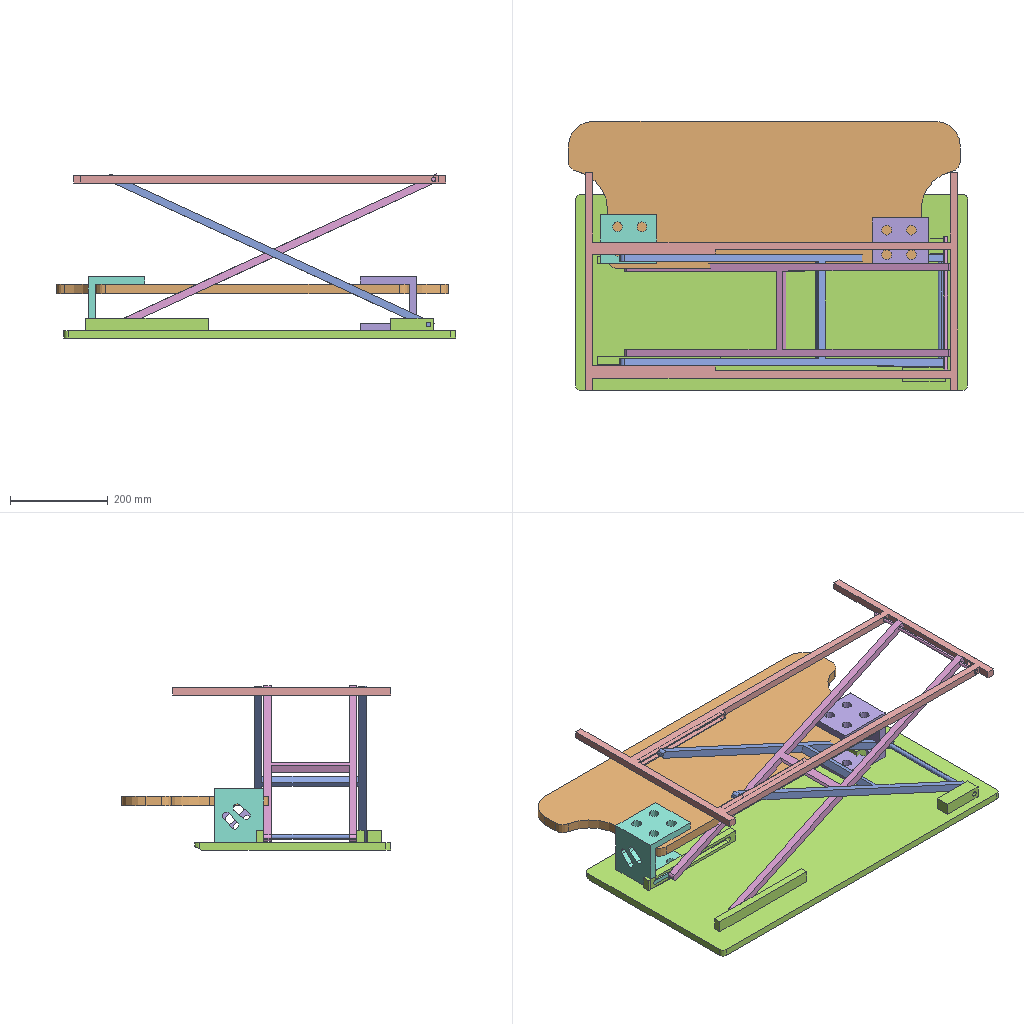Assembly | SolidWorks | 8 different items | 8 placed | box 815 x 549 x 335 mm
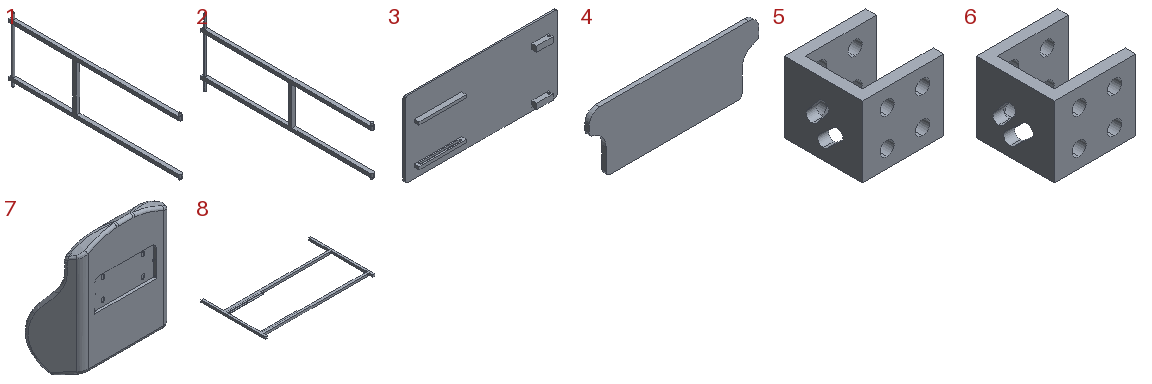Parts list (item | quantity | size | volume | features):
1 | x1 | 15 x 730 x 270 mm | 392693 mm3 | features ICE 5, Extrusion 1, Fillet 1
2 | x1 | 15 x 730 x 285 mm | 378111 mm3 | features ICE 5, Extrusion 1, Fillet 1
3 | x1 | 800 x 40 x 400.131 mm | 4882709 mm3 | features ICE 4, Cut 2, Fillet 2, MirrorPattern 2, Draft 1, Extrusion 1
4 | x1 | 800 x 20 x 300 mm | 4187582 mm3 | features Fillet 2, Extrusion 1
5 | x1 | 115 x 110 x 100 mm | 409059 mm3 | features ICE 2, Extrusion 1
6 | x1 | 115 x 110 x 100 mm | 406186 mm3 | features ICE 2, Extrusion 1
7 | x1 | 1267 x 391.764 x 1203 mm | 196548846 mm3 | features ICE 13, MirrorPattern 6, Fillet 5, Extrusion 1, RefAxis 1, Scale 1
8 | x1 | 760 x 445 x 15 mm | 540712 mm3 | features ICE 4, Cut 1, Extrusion 1
Mates (type | each side: item.copy, entity, surface, feature):
Parallel | 8.1 face plane Boss-Extrude1 | 3.1 face plane Boss-Extrude1
Width | 3.1 face plane Boss-Extrude1 | 3.1 face plane Boss-Extrude1 | 8.1 face plane Boss-Extrude1 | 8.1 face plane Boss-Extrude1
Parallel | 8.1 face plane Boss-Extrude5 | 1.1 face plane Boss-Extrude1
Coincident | 8.1 face plane Boss-Extrude5 | 1.1 face plane Boss-Extrude1
Coincident | 8.1 face plane Boss-Extrude1 | 3.1 face plane Boss-Extrude1
Width | 2.1 face plane Boss-Extrude4 | 2.1 face plane Boss-Extrude1 | 8.1 face plane Boss-Extrude2 | 8.1 face plane Boss-Extrude2
Width | 3.1 face plane Boss-Extrude2 | 3.1 face plane Boss-Extrude2 | 2.1 face cylinder Boss-Extrude5
Tangent | 3.1 face plane Cut-Extrude4 | 2.1 face cylinder Boss-Extrude5
Tangent | 8.1 face plane Boss-Extrude5 | 1.1 face cylinder Boss-Extrude2
Width | 8.1 face plane Boss-Extrude6 | 8.1 face plane Boss-Extrude1 | 1.1 face cylinder Boss-Extrude5
Concentric | 8.1 face cylinder Cut-Extrude2 | 2.1 face cylinder Boss-Extrude6
Concentric | 1.1 face cylinder Boss-Extrude6 | 3.1 face cylinder Cut-Extrude5
Coincident | 5.1 face plane Boss-Extrude1 | 4.1 face plane Boss-Extrude1 | 2 times
DistanceDim | 4.1 face plane Boss-Extrude1 | 5.1 face plane Boss-Extrude1
Coincident | 4.1 face plane Boss-Extrude1 | 6.1 face plane Boss-Extrude1 | 2 times
DistanceDim | 4.1 face plane Boss-Extrude1 | 6.1 face plane Boss-Extrude1
Coincident | 3.1 face plane Boss-Extrude1 | 5.1 face plane Boss-Extrude1
DistanceDim | 3.1 face plane Boss-Extrude1 | 5.1 face plane Boss-Extrude1